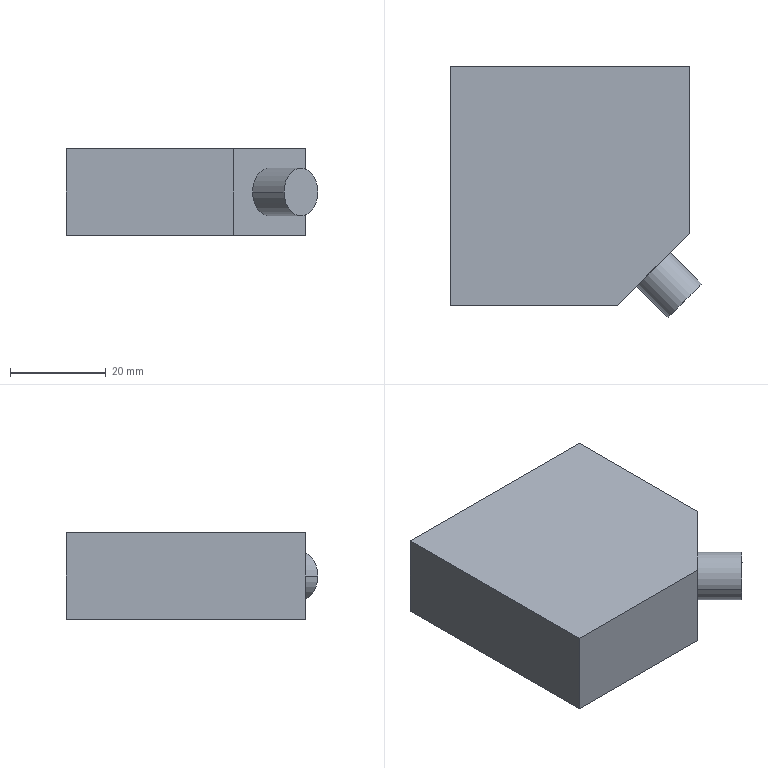Part | STEP file | Through-beam photoelectric sensor | 1 solid | 10 faces | box 52.612 x 52.612 x 18 mm | volume 43705 mm3 | plane 8 | cylinder 2 | commonest cylinder face diameters 10 x2
STEP:
#1=CARTESIAN_POINT('',(0.,0.,0.));
#2=DIRECTION('',(0.,0.,1.));
#3=DIRECTION('',(1.,0.,0.));
#4=AXIS2_PLACEMENT_3D('',#1,#2,#3);
#5=CARTESIAN_POINT('',(52.612,-45.541,9.));
#6=VERTEX_POINT('',#5);
#7=CARTESIAN_POINT('',(45.541,-52.612,9.));
#8=VERTEX_POINT('',#7);
#9=CARTESIAN_POINT('',(49.076,-49.076,9.));
#10=DIRECTION('',(0.7071,-0.7071,0.));
#11=DIRECTION('',(0.7071,0.7071,0.));
#12=AXIS2_PLACEMENT_3D('',#9,#10,#11);
#13=CIRCLE('',#12,5.);
#14=CARTESIAN_POINT('',(49.076,-49.076,9.));
#15=DIRECTION('',(-0.7071,0.7071,0.));
#16=DIRECTION('',(-0.7071,-0.7071,0.));
#17=AXIS2_PLACEMENT_3D('',#14,#15,#16);
#18=CYLINDRICAL_SURFACE('',#17,5.);
#19=CARTESIAN_POINT('',(3.142,0.));
#20=DIRECTION('',(-1.,0.));
#21=VECTOR('',#20,1.);
#22=LINE('',#19,#21);
#23=(GEOMETRIC_REPRESENTATION_CONTEXT(2)PARAMETRIC_REPRESENTATION_CONTEXT()REPRESENTATION_CONTEXT('',''));
#24=DEFINITIONAL_REPRESENTATION('',(#22),#23);
#25=PCURVE('',#18,#24);
#26=CARTESIAN_POINT('',(49.076,-49.076,9.));
#27=DIRECTION('',(0.7071,-0.7071,0.));
#28=DIRECTION('',(0.7071,0.7071,0.));
#29=AXIS2_PLACEMENT_3D('',#26,#27,#28);
#30=PLANE('',#29);
#31=CARTESIAN_POINT('',(0.,0.));
#32=DIRECTION('',(1.,0.));
#33=AXIS2_PLACEMENT_2D('',#31,#32);
#34=CIRCLE('',#33,5.);
#35=(GEOMETRIC_REPRESENTATION_CONTEXT(2)PARAMETRIC_REPRESENTATION_CONTEXT()REPRESENTATION_CONTEXT('',''));
#36=DEFINITIONAL_REPRESENTATION('',(#34),#35);
#37=PCURVE('',#30,#36);
#38=SURFACE_CURVE('',#13,(#25,#37),.PCURVE_S1.);
#39=EDGE_CURVE('',#6,#8,#38,.T.);
#40=ORIENTED_EDGE('',*,*,#39,.F.);
#41=CARTESIAN_POINT('',(46.036,-38.964,9.));
#42=VERTEX_POINT('',#41);
#43=CARTESIAN_POINT('',(52.612,-45.541,9.));
#44=DIRECTION('',(-0.7071,0.7071,0.));
#45=VECTOR('',#44,1.);
#46=LINE('',#43,#45);
#47=CARTESIAN_POINT('',(3.142,0.));
#48=DIRECTION('',(0.,1.));
#49=VECTOR('',#48,1.);
#50=LINE('',#47,#49);
#51=(GEOMETRIC_REPRESENTATION_CONTEXT(2)PARAMETRIC_REPRESENTATION_CONTEXT()REPRESENTATION_CONTEXT('',''));
#52=DEFINITIONAL_REPRESENTATION('',(#50),#51);
#53=PCURVE('',#18,#52);
#54=CARTESIAN_POINT('',(49.076,-49.076,9.));
#55=DIRECTION('',(-0.7071,0.7071,0.));
#56=DIRECTION('',(-0.7071,-0.7071,0.));
#57=AXIS2_PLACEMENT_3D('',#54,#55,#56);
#58=CYLINDRICAL_SURFACE('',#57,5.);
#59=CARTESIAN_POINT('',(3.142,0.));
#60=DIRECTION('',(0.,1.));
#61=VECTOR('',#60,1.);
#62=LINE('',#59,#61);
#63=(GEOMETRIC_REPRESENTATION_CONTEXT(2)PARAMETRIC_REPRESENTATION_CONTEXT()REPRESENTATION_CONTEXT('',''));
#64=DEFINITIONAL_REPRESENTATION('',(#62),#63);
#65=PCURVE('',#58,#64);
#66=SURFACE_CURVE('',#46,(#53,#65),.PCURVE_S1.);
#67=EDGE_CURVE('',#6,#42,#66,.T.);
#68=ORIENTED_EDGE('',*,*,#67,.T.);
#69=CARTESIAN_POINT('',(38.964,-46.036,9.));
#70=VERTEX_POINT('',#69);
#71=CARTESIAN_POINT('',(42.5,-42.5,9.));
#72=DIRECTION('',(0.7071,-0.7071,0.));
#73=DIRECTION('',(-0.7071,-0.7071,0.));
#74=AXIS2_PLACEMENT_3D('',#71,#72,#73);
#75=CIRCLE('',#74,5.);
#76=CARTESIAN_POINT('',(6.283,9.3));
#77=DIRECTION('',(-1.,0.));
#78=VECTOR('',#77,1.);
#79=LINE('',#76,#78);
#80=(GEOMETRIC_REPRESENTATION_CONTEXT(2)PARAMETRIC_REPRESENTATION_CONTEXT()REPRESENTATION_CONTEXT('',''));
#81=DEFINITIONAL_REPRESENTATION('',(#79),#80);
#82=PCURVE('',#18,#81);
#83=CARTESIAN_POINT('',(35.,-50.,18.));
#84=DIRECTION('',(-0.7071,0.7071,0.));
#85=DIRECTION('',(-0.7071,-0.7071,0.));
#86=AXIS2_PLACEMENT_3D('',#83,#84,#85);
#87=PLANE('',#86);
#88=CARTESIAN_POINT('',(-5.607,-9.));
#89=CARTESIAN_POINT('',(-5.607,-17.66));
#90=CARTESIAN_POINT('',(-13.107,-13.33));
#91=CARTESIAN_POINT('',(-20.607,-9.));
#92=CARTESIAN_POINT('',(-13.107,-4.67));
#93=CARTESIAN_POINT('',(-5.607,-0.3397));
#94=CARTESIAN_POINT('',(-5.607,-9.));
#95=(BOUNDED_CURVE()B_SPLINE_CURVE(2,(#88,#89,#90,#91,#92,#93,#94),.UNSPECIFIED.,.T.,.F.)B_SPLINE_CURVE_WITH_KNOTS((1,2,2,2,2,1),(-2.094,0.,2.094,4.189,6.283,8.378),.UNSPECIFIED.)CURVE()GEOMETRIC_REPRESENTATION_ITEM()RATIONAL_B_SPLINE_CURVE((1.,0.5,1.,0.5,1.,0.5,1.))REPRESENTATION_ITEM(''));
#96=(GEOMETRIC_REPRESENTATION_CONTEXT(2)PARAMETRIC_REPRESENTATION_CONTEXT()REPRESENTATION_CONTEXT('',''));
#97=DEFINITIONAL_REPRESENTATION('',(#95),#96);
#98=PCURVE('',#87,#97);
#99=SURFACE_CURVE('',#75,(#82,#98),.PCURVE_S1.);
#100=EDGE_CURVE('',#42,#70,#99,.T.);
#101=ORIENTED_EDGE('',*,*,#100,.T.);
#102=CARTESIAN_POINT('',(45.541,-52.612,9.));
#103=DIRECTION('',(-0.7071,0.7071,0.));
#104=VECTOR('',#103,1.);
#105=LINE('',#102,#104);
#106=CARTESIAN_POINT('',(0.,0.));
#107=DIRECTION('',(0.,1.));
#108=VECTOR('',#107,1.);
#109=LINE('',#106,#108);
#110=(GEOMETRIC_REPRESENTATION_CONTEXT(2)PARAMETRIC_REPRESENTATION_CONTEXT()REPRESENTATION_CONTEXT('',''));
#111=DEFINITIONAL_REPRESENTATION('',(#109),#110);
#112=PCURVE('',#18,#111);
#113=CARTESIAN_POINT('',(6.283,0.));
#114=DIRECTION('',(0.,1.));
#115=VECTOR('',#114,1.);
#116=LINE('',#113,#115);
#117=(GEOMETRIC_REPRESENTATION_CONTEXT(2)PARAMETRIC_REPRESENTATION_CONTEXT()REPRESENTATION_CONTEXT('',''));
#118=DEFINITIONAL_REPRESENTATION('',(#116),#117);
#119=PCURVE('',#58,#118);
#120=SURFACE_CURVE('',#105,(#112,#119),.PCURVE_S1.);
#121=EDGE_CURVE('',#8,#70,#120,.T.);
#122=ORIENTED_EDGE('',*,*,#121,.F.);
#123=EDGE_LOOP('',(#40,#68,#101,#122));
#124=FACE_BOUND('',#123,.T.);
#125=ADVANCED_FACE('',(#124),#18,.T.);
#126=CARTESIAN_POINT('',(35.,-50.,0.));
#127=VERTEX_POINT('',#126);
#128=CARTESIAN_POINT('',(50.,-35.,0.));
#129=VERTEX_POINT('',#128);
#130=CARTESIAN_POINT('',(35.,-50.,0.));
#131=DIRECTION('',(0.7071,0.7071,0.));
#132=VECTOR('',#131,1.);
#133=LINE('',#130,#132);
#134=CARTESIAN_POINT('',(0.,-18.));
#135=DIRECTION('',(-1.,0.));
#136=VECTOR('',#135,1.);
#137=LINE('',#134,#136);
#138=(GEOMETRIC_REPRESENTATION_CONTEXT(2)PARAMETRIC_REPRESENTATION_CONTEXT()REPRESENTATION_CONTEXT('',''));
#139=DEFINITIONAL_REPRESENTATION('',(#137),#138);
#140=PCURVE('',#87,#139);
#141=CARTESIAN_POINT('',(0.,0.,0.));
#142=DIRECTION('',(0.,0.,1.));
#143=DIRECTION('',(1.,0.,0.));
#144=AXIS2_PLACEMENT_3D('',#141,#142,#143);
#145=PLANE('',#144);
#146=CARTESIAN_POINT('',(35.,-50.));
#147=DIRECTION('',(0.7071,0.7071));
#148=VECTOR('',#147,1.);
#149=LINE('',#146,#148);
#150=(GEOMETRIC_REPRESENTATION_CONTEXT(2)PARAMETRIC_REPRESENTATION_CONTEXT()REPRESENTATION_CONTEXT('',''));
#151=DEFINITIONAL_REPRESENTATION('',(#149),#150);
#152=PCURVE('',#145,#151);
#153=SURFACE_CURVE('',#133,(#140,#152),.PCURVE_S1.);
#154=EDGE_CURVE('',#127,#129,#153,.T.);
#155=ORIENTED_EDGE('',*,*,#154,.T.);
#156=CARTESIAN_POINT('',(50.,-35.,18.));
#157=VERTEX_POINT('',#156);
#158=CARTESIAN_POINT('',(50.,-35.,18.));
#159=DIRECTION('',(0.,0.,-1.));
#160=VECTOR('',#159,1.);
#161=LINE('',#158,#160);
#162=CARTESIAN_POINT('',(-21.213,0.));
#163=DIRECTION('',(0.,-1.));
#164=VECTOR('',#163,1.);
#165=LINE('',#162,#164);
#166=(GEOMETRIC_REPRESENTATION_CONTEXT(2)PARAMETRIC_REPRESENTATION_CONTEXT()REPRESENTATION_CONTEXT('',''));
#167=DEFINITIONAL_REPRESENTATION('',(#165),#166);
#168=PCURVE('',#87,#167);
#169=CARTESIAN_POINT('',(50.,0.,18.));
#170=DIRECTION('',(-1.,0.,0.));
#171=DIRECTION('',(0.,-1.,0.));
#172=AXIS2_PLACEMENT_3D('',#169,#170,#171);
#173=PLANE('',#172);
#174=CARTESIAN_POINT('',(35.,0.));
#175=DIRECTION('',(0.,-1.));
#176=VECTOR('',#175,1.);
#177=LINE('',#174,#176);
#178=(GEOMETRIC_REPRESENTATION_CONTEXT(2)PARAMETRIC_REPRESENTATION_CONTEXT()REPRESENTATION_CONTEXT('',''));
#179=DEFINITIONAL_REPRESENTATION('',(#177),#178);
#180=PCURVE('',#173,#179);
#181=SURFACE_CURVE('',#161,(#168,#180),.PCURVE_S1.);
#182=EDGE_CURVE('',#157,#129,#181,.T.);
#183=ORIENTED_EDGE('',*,*,#182,.F.);
#184=CARTESIAN_POINT('',(35.,-50.,18.));
#185=VERTEX_POINT('',#184);
#186=CARTESIAN_POINT('',(35.,-50.,18.));
#187=DIRECTION('',(0.7071,0.7071,0.));
#188=VECTOR('',#187,1.);
#189=LINE('',#186,#188);
#190=CARTESIAN_POINT('',(0.,0.));
#191=DIRECTION('',(-1.,0.));
#192=VECTOR('',#191,1.);
#193=LINE('',#190,#192);
#194=(GEOMETRIC_REPRESENTATION_CONTEXT(2)PARAMETRIC_REPRESENTATION_CONTEXT()REPRESENTATION_CONTEXT('',''));
#195=DEFINITIONAL_REPRESENTATION('',(#193),#194);
#196=PCURVE('',#87,#195);
#197=CARTESIAN_POINT('',(0.,0.,18.));
#198=DIRECTION('',(0.,0.,1.));
#199=DIRECTION('',(1.,0.,0.));
#200=AXIS2_PLACEMENT_3D('',#197,#198,#199);
#201=PLANE('',#200);
#202=CARTESIAN_POINT('',(35.,-50.));
#203=DIRECTION('',(0.7071,0.7071));
#204=VECTOR('',#203,1.);
#205=LINE('',#202,#204);
#206=(GEOMETRIC_REPRESENTATION_CONTEXT(2)PARAMETRIC_REPRESENTATION_CONTEXT()REPRESENTATION_CONTEXT('',''));
#207=DEFINITIONAL_REPRESENTATION('',(#205),#206);
#208=PCURVE('',#201,#207);
#209=SURFACE_CURVE('',#189,(#196,#208),.PCURVE_S1.);
#210=EDGE_CURVE('',#185,#157,#209,.T.);
#211=ORIENTED_EDGE('',*,*,#210,.F.);
#212=CARTESIAN_POINT('',(35.,-50.,18.));
#213=DIRECTION('',(0.,0.,-1.));
#214=VECTOR('',#213,1.);
#215=LINE('',#212,#214);
#216=CARTESIAN_POINT('',(0.,0.));
#217=DIRECTION('',(0.,-1.));
#218=VECTOR('',#217,1.);
#219=LINE('',#216,#218);
#220=(GEOMETRIC_REPRESENTATION_CONTEXT(2)PARAMETRIC_REPRESENTATION_CONTEXT()REPRESENTATION_CONTEXT('',''));
#221=DEFINITIONAL_REPRESENTATION('',(#219),#220);
#222=PCURVE('',#87,#221);
#223=CARTESIAN_POINT('',(0.,-50.,18.));
#224=DIRECTION('',(0.,1.,0.));
#225=DIRECTION('',(0.,0.,1.));
#226=AXIS2_PLACEMENT_3D('',#223,#224,#225);
#227=PLANE('',#226);
#228=CARTESIAN_POINT('',(0.,35.));
#229=DIRECTION('',(-1.,0.));
#230=VECTOR('',#229,1.);
#231=LINE('',#228,#230);
#232=(GEOMETRIC_REPRESENTATION_CONTEXT(2)PARAMETRIC_REPRESENTATION_CONTEXT()REPRESENTATION_CONTEXT('',''));
#233=DEFINITIONAL_REPRESENTATION('',(#231),#232);
#234=PCURVE('',#227,#233);
#235=SURFACE_CURVE('',#215,(#222,#234),.PCURVE_S1.);
#236=EDGE_CURVE('',#185,#127,#235,.T.);
#237=ORIENTED_EDGE('',*,*,#236,.T.);
#238=EDGE_LOOP('',(#155,#183,#211,#237));
#239=FACE_BOUND('',#238,.T.);
#240=CARTESIAN_POINT('',(42.5,-42.5,9.));
#241=DIRECTION('',(0.7071,-0.7071,0.));
#242=DIRECTION('',(-0.7071,-0.7071,0.));
#243=AXIS2_PLACEMENT_3D('',#240,#241,#242);
#244=CIRCLE('',#243,5.);
#245=CARTESIAN_POINT('',(-5.607,-9.));
#246=CARTESIAN_POINT('',(-5.607,-17.66));
#247=CARTESIAN_POINT('',(-13.107,-13.33));
#248=CARTESIAN_POINT('',(-20.607,-9.));
#249=CARTESIAN_POINT('',(-13.107,-4.67));
#250=CARTESIAN_POINT('',(-5.607,-0.3397));
#251=CARTESIAN_POINT('',(-5.607,-9.));
#252=(BOUNDED_CURVE()B_SPLINE_CURVE(2,(#245,#246,#247,#248,#249,#250,#251),.UNSPECIFIED.,.T.,.F.)B_SPLINE_CURVE_WITH_KNOTS((1,2,2,2,2,1),(-2.094,0.,2.094,4.189,6.283,8.378),.UNSPECIFIED.)CURVE()GEOMETRIC_REPRESENTATION_ITEM()RATIONAL_B_SPLINE_CURVE((1.,0.5,1.,0.5,1.,0.5,1.))REPRESENTATION_ITEM(''));
#253=(GEOMETRIC_REPRESENTATION_CONTEXT(2)PARAMETRIC_REPRESENTATION_CONTEXT()REPRESENTATION_CONTEXT('',''));
#254=DEFINITIONAL_REPRESENTATION('',(#252),#253);
#255=PCURVE('',#87,#254);
#256=CARTESIAN_POINT('',(6.283,9.3));
#257=DIRECTION('',(-1.,0.));
#258=VECTOR('',#257,1.);
#259=LINE('',#256,#258);
#260=(GEOMETRIC_REPRESENTATION_CONTEXT(2)PARAMETRIC_REPRESENTATION_CONTEXT()REPRESENTATION_CONTEXT('',''));
#261=DEFINITIONAL_REPRESENTATION('',(#259),#260);
#262=PCURVE('',#58,#261);
#263=SURFACE_CURVE('',#244,(#255,#262),.PCURVE_S1.);
#264=EDGE_CURVE('',#70,#42,#263,.T.);
#265=ORIENTED_EDGE('',*,*,#264,.F.);
#266=ORIENTED_EDGE('',*,*,#100,.F.);
#267=EDGE_LOOP('',(#265,#266));
#268=FACE_BOUND('',#267,.T.);
#269=ADVANCED_FACE('',(#239,#268),#87,.F.);
#270=CARTESIAN_POINT('',(0.,0.,0.));
#271=VERTEX_POINT('',#270);
#272=CARTESIAN_POINT('',(0.,-50.,0.));
#273=VERTEX_POINT('',#272);
#274=CARTESIAN_POINT('',(0.,0.,0.));
#275=DIRECTION('',(0.,-1.,0.));
#276=VECTOR('',#275,1.);
#277=LINE('',#274,#276);
#278=CARTESIAN_POINT('',(0.,0.,18.));
#279=DIRECTION('',(1.,0.,0.));
#280=DIRECTION('',(0.,1.,0.));
#281=AXIS2_PLACEMENT_3D('',#278,#279,#280);
#282=PLANE('',#281);
#283=CARTESIAN_POINT('',(0.,-18.));
#284=DIRECTION('',(-1.,0.));
#285=VECTOR('',#284,1.);
#286=LINE('',#283,#285);
#287=(GEOMETRIC_REPRESENTATION_CONTEXT(2)PARAMETRIC_REPRESENTATION_CONTEXT()REPRESENTATION_CONTEXT('',''));
#288=DEFINITIONAL_REPRESENTATION('',(#286),#287);
#289=PCURVE('',#282,#288);
#290=CARTESIAN_POINT('',(0.,0.));
#291=DIRECTION('',(0.,-1.));
#292=VECTOR('',#291,1.);
#293=LINE('',#290,#292);
#294=(GEOMETRIC_REPRESENTATION_CONTEXT(2)PARAMETRIC_REPRESENTATION_CONTEXT()REPRESENTATION_CONTEXT('',''));
#295=DEFINITIONAL_REPRESENTATION('',(#293),#294);
#296=PCURVE('',#145,#295);
#297=SURFACE_CURVE('',#277,(#289,#296),.PCURVE_S1.);
#298=EDGE_CURVE('',#271,#273,#297,.T.);
#299=ORIENTED_EDGE('',*,*,#298,.T.);
#300=CARTESIAN_POINT('',(0.,-50.,18.));
#301=VERTEX_POINT('',#300);
#302=CARTESIAN_POINT('',(0.,-50.,18.));
#303=DIRECTION('',(0.,0.,-1.));
#304=VECTOR('',#303,1.);
#305=LINE('',#302,#304);
#306=CARTESIAN_POINT('',(-50.,0.));
#307=DIRECTION('',(0.,-1.));
#308=VECTOR('',#307,1.);
#309=LINE('',#306,#308);
#310=(GEOMETRIC_REPRESENTATION_CONTEXT(2)PARAMETRIC_REPRESENTATION_CONTEXT()REPRESENTATION_CONTEXT('',''));
#311=DEFINITIONAL_REPRESENTATION('',(#309),#310);
#312=PCURVE('',#282,#311);
#313=CARTESIAN_POINT('',(0.,0.));
#314=DIRECTION('',(-1.,0.));
#315=VECTOR('',#314,1.);
#316=LINE('',#313,#315);
#317=(GEOMETRIC_REPRESENTATION_CONTEXT(2)PARAMETRIC_REPRESENTATION_CONTEXT()REPRESENTATION_CONTEXT('',''));
#318=DEFINITIONAL_REPRESENTATION('',(#316),#317);
#319=PCURVE('',#227,#318);
#320=SURFACE_CURVE('',#305,(#312,#319),.PCURVE_S1.);
#321=EDGE_CURVE('',#301,#273,#320,.T.);
#322=ORIENTED_EDGE('',*,*,#321,.F.);
#323=CARTESIAN_POINT('',(0.,0.,18.));
#324=VERTEX_POINT('',#323);
#325=CARTESIAN_POINT('',(0.,0.,18.));
#326=DIRECTION('',(0.,-1.,0.));
#327=VECTOR('',#326,1.);
#328=LINE('',#325,#327);
#329=CARTESIAN_POINT('',(0.,0.));
#330=DIRECTION('',(-1.,0.));
#331=VECTOR('',#330,1.);
#332=LINE('',#329,#331);
#333=(GEOMETRIC_REPRESENTATION_CONTEXT(2)PARAMETRIC_REPRESENTATION_CONTEXT()REPRESENTATION_CONTEXT('',''));
#334=DEFINITIONAL_REPRESENTATION('',(#332),#333);
#335=PCURVE('',#282,#334);
#336=CARTESIAN_POINT('',(0.,0.));
#337=DIRECTION('',(0.,-1.));
#338=VECTOR('',#337,1.);
#339=LINE('',#336,#338);
#340=(GEOMETRIC_REPRESENTATION_CONTEXT(2)PARAMETRIC_REPRESENTATION_CONTEXT()REPRESENTATION_CONTEXT('',''));
#341=DEFINITIONAL_REPRESENTATION('',(#339),#340);
#342=PCURVE('',#201,#341);
#343=SURFACE_CURVE('',#328,(#335,#342),.PCURVE_S1.);
#344=EDGE_CURVE('',#324,#301,#343,.T.);
#345=ORIENTED_EDGE('',*,*,#344,.F.);
#346=CARTESIAN_POINT('',(0.,0.,18.));
#347=DIRECTION('',(0.,0.,-1.));
#348=VECTOR('',#347,1.);
#349=LINE('',#346,#348);
#350=CARTESIAN_POINT('',(0.,0.));
#351=DIRECTION('',(0.,-1.));
#352=VECTOR('',#351,1.);
#353=LINE('',#350,#352);
#354=(GEOMETRIC_REPRESENTATION_CONTEXT(2)PARAMETRIC_REPRESENTATION_CONTEXT()REPRESENTATION_CONTEXT('',''));
#355=DEFINITIONAL_REPRESENTATION('',(#353),#354);
#356=PCURVE('',#282,#355);
#357=CARTESIAN_POINT('',(0.,0.,18.));
#358=DIRECTION('',(0.,-1.,0.));
#359=DIRECTION('',(0.,0.,-1.));
#360=AXIS2_PLACEMENT_3D('',#357,#358,#359);
#361=PLANE('',#360);
#362=CARTESIAN_POINT('',(0.,0.));
#363=DIRECTION('',(1.,0.));
#364=VECTOR('',#363,1.);
#365=LINE('',#362,#364);
#366=(GEOMETRIC_REPRESENTATION_CONTEXT(2)PARAMETRIC_REPRESENTATION_CONTEXT()REPRESENTATION_CONTEXT('',''));
#367=DEFINITIONAL_REPRESENTATION('',(#365),#366);
#368=PCURVE('',#361,#367);
#369=SURFACE_CURVE('',#349,(#356,#368),.PCURVE_S1.);
#370=EDGE_CURVE('',#324,#271,#369,.T.);
#371=ORIENTED_EDGE('',*,*,#370,.T.);
#372=EDGE_LOOP('',(#299,#322,#345,#371));
#373=FACE_BOUND('',#372,.T.);
#374=ADVANCED_FACE('',(#373),#282,.F.);
#375=CARTESIAN_POINT('',(0.,-50.,0.));
#376=DIRECTION('',(1.,0.,0.));
#377=VECTOR('',#376,1.);
#378=LINE('',#375,#377);
#379=CARTESIAN_POINT('',(-18.,0.));
#380=DIRECTION('',(0.,1.));
#381=VECTOR('',#380,1.);
#382=LINE('',#379,#381);
#383=(GEOMETRIC_REPRESENTATION_CONTEXT(2)PARAMETRIC_REPRESENTATION_CONTEXT()REPRESENTATION_CONTEXT('',''));
#384=DEFINITIONAL_REPRESENTATION('',(#382),#383);
#385=PCURVE('',#227,#384);
#386=CARTESIAN_POINT('',(0.,-50.));
#387=DIRECTION('',(1.,0.));
#388=VECTOR('',#387,1.);
#389=LINE('',#386,#388);
#390=(GEOMETRIC_REPRESENTATION_CONTEXT(2)PARAMETRIC_REPRESENTATION_CONTEXT()REPRESENTATION_CONTEXT('',''));
#391=DEFINITIONAL_REPRESENTATION('',(#389),#390);
#392=PCURVE('',#145,#391);
#393=SURFACE_CURVE('',#378,(#385,#392),.PCURVE_S1.);
#394=EDGE_CURVE('',#273,#127,#393,.T.);
#395=ORIENTED_EDGE('',*,*,#394,.T.);
#396=ORIENTED_EDGE('',*,*,#236,.F.);
#397=CARTESIAN_POINT('',(0.,-50.,18.));
#398=DIRECTION('',(1.,0.,0.));
#399=VECTOR('',#398,1.);
#400=LINE('',#397,#399);
#401=CARTESIAN_POINT('',(0.,0.));
#402=DIRECTION('',(0.,1.));
#403=VECTOR('',#402,1.);
#404=LINE('',#401,#403);
#405=(GEOMETRIC_REPRESENTATION_CONTEXT(2)PARAMETRIC_REPRESENTATION_CONTEXT()REPRESENTATION_CONTEXT('',''));
#406=DEFINITIONAL_REPRESENTATION('',(#404),#405);
#407=PCURVE('',#227,#406);
#408=CARTESIAN_POINT('',(0.,-50.));
#409=DIRECTION('',(1.,0.));
#410=VECTOR('',#409,1.);
#411=LINE('',#408,#410);
#412=(GEOMETRIC_REPRESENTATION_CONTEXT(2)PARAMETRIC_REPRESENTATION_CONTEXT()REPRESENTATION_CONTEXT('',''));
#413=DEFINITIONAL_REPRESENTATION('',(#411),#412);
#414=PCURVE('',#201,#413);
#415=SURFACE_CURVE('',#400,(#407,#414),.PCURVE_S1.);
#416=EDGE_CURVE('',#301,#185,#415,.T.);
#417=ORIENTED_EDGE('',*,*,#416,.F.);
#418=ORIENTED_EDGE('',*,*,#321,.T.);
#419=EDGE_LOOP('',(#395,#396,#417,#418));
#420=FACE_BOUND('',#419,.T.);
#421=ADVANCED_FACE('',(#420),#227,.F.);
#422=CARTESIAN_POINT('',(50.,0.,0.));
#423=VERTEX_POINT('',#422);
#424=CARTESIAN_POINT('',(50.,0.,0.));
#425=DIRECTION('',(0.,1.,0.));
#426=VECTOR('',#425,1.);
#427=LINE('',#424,#426);
#428=CARTESIAN_POINT('',(0.,-18.));
#429=DIRECTION('',(-1.,0.));
#430=VECTOR('',#429,1.);
#431=LINE('',#428,#430);
#432=(GEOMETRIC_REPRESENTATION_CONTEXT(2)PARAMETRIC_REPRESENTATION_CONTEXT()REPRESENTATION_CONTEXT('',''));
#433=DEFINITIONAL_REPRESENTATION('',(#431),#432);
#434=PCURVE('',#173,#433);
#435=CARTESIAN_POINT('',(50.,0.));
#436=DIRECTION('',(0.,1.));
#437=VECTOR('',#436,1.);
#438=LINE('',#435,#437);
#439=(GEOMETRIC_REPRESENTATION_CONTEXT(2)PARAMETRIC_REPRESENTATION_CONTEXT()REPRESENTATION_CONTEXT('',''));
#440=DEFINITIONAL_REPRESENTATION('',(#438),#439);
#441=PCURVE('',#145,#440);
#442=SURFACE_CURVE('',#427,(#434,#441),.PCURVE_S1.);
#443=EDGE_CURVE('',#129,#423,#442,.T.);
#444=ORIENTED_EDGE('',*,*,#443,.T.);
#445=CARTESIAN_POINT('',(50.,0.,18.));
#446=VERTEX_POINT('',#445);
#447=CARTESIAN_POINT('',(50.,0.,18.));
#448=DIRECTION('',(0.,0.,-1.));
#449=VECTOR('',#448,1.);
#450=LINE('',#447,#449);
#451=CARTESIAN_POINT('',(0.,0.));
#452=DIRECTION('',(0.,-1.));
#453=VECTOR('',#452,1.);
#454=LINE('',#451,#453);
#455=(GEOMETRIC_REPRESENTATION_CONTEXT(2)PARAMETRIC_REPRESENTATION_CONTEXT()REPRESENTATION_CONTEXT('',''));
#456=DEFINITIONAL_REPRESENTATION('',(#454),#455);
#457=PCURVE('',#173,#456);
#458=CARTESIAN_POINT('',(0.,50.));
#459=DIRECTION('',(1.,0.));
#460=VECTOR('',#459,1.);
#461=LINE('',#458,#460);
#462=(GEOMETRIC_REPRESENTATION_CONTEXT(2)PARAMETRIC_REPRESENTATION_CONTEXT()REPRESENTATION_CONTEXT('',''));
#463=DEFINITIONAL_REPRESENTATION('',(#461),#462);
#464=PCURVE('',#361,#463);
#465=SURFACE_CURVE('',#450,(#457,#464),.PCURVE_S1.);
#466=EDGE_CURVE('',#446,#423,#465,.T.);
#467=ORIENTED_EDGE('',*,*,#466,.F.);
#468=CARTESIAN_POINT('',(50.,0.,18.));
#469=DIRECTION('',(0.,1.,0.));
#470=VECTOR('',#469,1.);
#471=LINE('',#468,#470);
#472=CARTESIAN_POINT('',(0.,0.));
#473=DIRECTION('',(-1.,0.));
#474=VECTOR('',#473,1.);
#475=LINE('',#472,#474);
#476=(GEOMETRIC_REPRESENTATION_CONTEXT(2)PARAMETRIC_REPRESENTATION_CONTEXT()REPRESENTATION_CONTEXT('',''));
#477=DEFINITIONAL_REPRESENTATION('',(#475),#476);
#478=PCURVE('',#173,#477);
#479=CARTESIAN_POINT('',(50.,0.));
#480=DIRECTION('',(0.,1.));
#481=VECTOR('',#480,1.);
#482=LINE('',#479,#481);
#483=(GEOMETRIC_REPRESENTATION_CONTEXT(2)PARAMETRIC_REPRESENTATION_CONTEXT()REPRESENTATION_CONTEXT('',''));
#484=DEFINITIONAL_REPRESENTATION('',(#482),#483);
#485=PCURVE('',#201,#484);
#486=SURFACE_CURVE('',#471,(#478,#485),.PCURVE_S1.);
#487=EDGE_CURVE('',#157,#446,#486,.T.);
#488=ORIENTED_EDGE('',*,*,#487,.F.);
#489=ORIENTED_EDGE('',*,*,#182,.T.);
#490=EDGE_LOOP('',(#444,#467,#488,#489));
#491=FACE_BOUND('',#490,.T.);
#492=ADVANCED_FACE('',(#491),#173,.F.);
#493=CARTESIAN_POINT('',(0.,0.,0.));
#494=DIRECTION('',(-1.,0.,0.));
#495=VECTOR('',#494,1.);
#496=LINE('',#493,#495);
#497=CARTESIAN_POINT('',(18.,0.));
#498=DIRECTION('',(0.,-1.));
#499=VECTOR('',#498,1.);
#500=LINE('',#497,#499);
#501=(GEOMETRIC_REPRESENTATION_CONTEXT(2)PARAMETRIC_REPRESENTATION_CONTEXT()REPRESENTATION_CONTEXT('',''));
#502=DEFINITIONAL_REPRESENTATION('',(#500),#501);
#503=PCURVE('',#361,#502);
#504=CARTESIAN_POINT('',(0.,0.));
#505=DIRECTION('',(-1.,0.));
#506=VECTOR('',#505,1.);
#507=LINE('',#504,#506);
#508=(GEOMETRIC_REPRESENTATION_CONTEXT(2)PARAMETRIC_REPRESENTATION_CONTEXT()REPRESENTATION_CONTEXT('',''));
#509=DEFINITIONAL_REPRESENTATION('',(#507),#508);
#510=PCURVE('',#145,#509);
#511=SURFACE_CURVE('',#496,(#503,#510),.PCURVE_S1.);
#512=EDGE_CURVE('',#423,#271,#511,.T.);
#513=ORIENTED_EDGE('',*,*,#512,.T.);
#514=ORIENTED_EDGE('',*,*,#370,.F.);
#515=CARTESIAN_POINT('',(0.,0.,18.));
#516=DIRECTION('',(-1.,0.,0.));
#517=VECTOR('',#516,1.);
#518=LINE('',#515,#517);
#519=CARTESIAN_POINT('',(0.,0.));
#520=DIRECTION('',(0.,-1.));
#521=VECTOR('',#520,1.);
#522=LINE('',#519,#521);
#523=(GEOMETRIC_REPRESENTATION_CONTEXT(2)PARAMETRIC_REPRESENTATION_CONTEXT()REPRESENTATION_CONTEXT('',''));
#524=DEFINITIONAL_REPRESENTATION('',(#522),#523);
#525=PCURVE('',#361,#524);
#526=CARTESIAN_POINT('',(0.,0.));
#527=DIRECTION('',(-1.,0.));
#528=VECTOR('',#527,1.);
#529=LINE('',#526,#528);
#530=(GEOMETRIC_REPRESENTATION_CONTEXT(2)PARAMETRIC_REPRESENTATION_CONTEXT()REPRESENTATION_CONTEXT('',''));
#531=DEFINITIONAL_REPRESENTATION('',(#529),#530);
#532=PCURVE('',#201,#531);
#533=SURFACE_CURVE('',#518,(#525,#532),.PCURVE_S1.);
#534=EDGE_CURVE('',#446,#324,#533,.T.);
#535=ORIENTED_EDGE('',*,*,#534,.F.);
#536=ORIENTED_EDGE('',*,*,#466,.T.);
#537=EDGE_LOOP('',(#513,#514,#535,#536));
#538=FACE_BOUND('',#537,.T.);
#539=ADVANCED_FACE('',(#538),#361,.F.);
#540=ORIENTED_EDGE('',*,*,#344,.T.);
#541=ORIENTED_EDGE('',*,*,#416,.T.);
#542=ORIENTED_EDGE('',*,*,#210,.T.);
#543=ORIENTED_EDGE('',*,*,#487,.T.);
#544=ORIENTED_EDGE('',*,*,#534,.T.);
#545=EDGE_LOOP('',(#540,#541,#542,#543,#544));
#546=FACE_BOUND('',#545,.T.);
#547=ADVANCED_FACE('',(#546),#201,.T.);
#548=ORIENTED_EDGE('',*,*,#298,.F.);
#549=ORIENTED_EDGE('',*,*,#512,.F.);
#550=ORIENTED_EDGE('',*,*,#443,.F.);
#551=ORIENTED_EDGE('',*,*,#154,.F.);
#552=ORIENTED_EDGE('',*,*,#394,.F.);
#553=EDGE_LOOP('',(#548,#549,#550,#551,#552));
#554=FACE_BOUND('',#553,.T.);
#555=ADVANCED_FACE('',(#554),#145,.F.);
#556=ORIENTED_EDGE('',*,*,#67,.F.);
#557=CARTESIAN_POINT('',(49.076,-49.076,9.));
#558=DIRECTION('',(0.7071,-0.7071,0.));
#559=DIRECTION('',(0.7071,0.7071,0.));
#560=AXIS2_PLACEMENT_3D('',#557,#558,#559);
#561=CIRCLE('',#560,5.);
#562=CARTESIAN_POINT('',(9.425,0.));
#563=DIRECTION('',(-1.,0.));
#564=VECTOR('',#563,1.);
#565=LINE('',#562,#564);
#566=(GEOMETRIC_REPRESENTATION_CONTEXT(2)PARAMETRIC_REPRESENTATION_CONTEXT()REPRESENTATION_CONTEXT('',''));
#567=DEFINITIONAL_REPRESENTATION('',(#565),#566);
#568=PCURVE('',#58,#567);
#569=CARTESIAN_POINT('',(0.,0.));
#570=DIRECTION('',(1.,0.));
#571=AXIS2_PLACEMENT_2D('',#569,#570);
#572=CIRCLE('',#571,5.);
#573=(GEOMETRIC_REPRESENTATION_CONTEXT(2)PARAMETRIC_REPRESENTATION_CONTEXT()REPRESENTATION_CONTEXT('',''));
#574=DEFINITIONAL_REPRESENTATION('',(#572),#573);
#575=PCURVE('',#30,#574);
#576=SURFACE_CURVE('',#561,(#568,#575),.PCURVE_S1.);
#577=EDGE_CURVE('',#8,#6,#576,.T.);
#578=ORIENTED_EDGE('',*,*,#577,.F.);
#579=ORIENTED_EDGE('',*,*,#121,.T.);
#580=ORIENTED_EDGE('',*,*,#264,.T.);
#581=EDGE_LOOP('',(#556,#578,#579,#580));
#582=FACE_BOUND('',#581,.T.);
#583=ADVANCED_FACE('',(#582),#58,.T.);
#584=ORIENTED_EDGE('',*,*,#577,.T.);
#585=ORIENTED_EDGE('',*,*,#39,.T.);
#586=EDGE_LOOP('',(#584,#585));
#587=FACE_BOUND('',#586,.T.);
#588=ADVANCED_FACE('',(#587),#30,.T.);
#589=CLOSED_SHELL('',(#125,#269,#374,#421,#492,#539,#547,#555,#583,#588));
#590=MANIFOLD_SOLID_BREP('',#589);
#591=(LENGTH_UNIT()NAMED_UNIT(*)SI_UNIT(.MILLI.,.METRE.));
#592=UNCERTAINTY_MEASURE_WITH_UNIT(LENGTH_MEASURE(0.0000001),#591,'','');
#593=(NAMED_UNIT(*)PLANE_ANGLE_UNIT()SI_UNIT($,.RADIAN.));
#594=(NAMED_UNIT(*)SI_UNIT($,.STERADIAN.)SOLID_ANGLE_UNIT());
#595=(GEOMETRIC_REPRESENTATION_CONTEXT(3)GLOBAL_UNCERTAINTY_ASSIGNED_CONTEXT((#592))GLOBAL_UNIT_ASSIGNED_CONTEXT((#591,#593,#594))REPRESENTATION_CONTEXT('',''));
#596=ADVANCED_BREP_SHAPE_REPRESENTATION('',(#4,#590),#595);